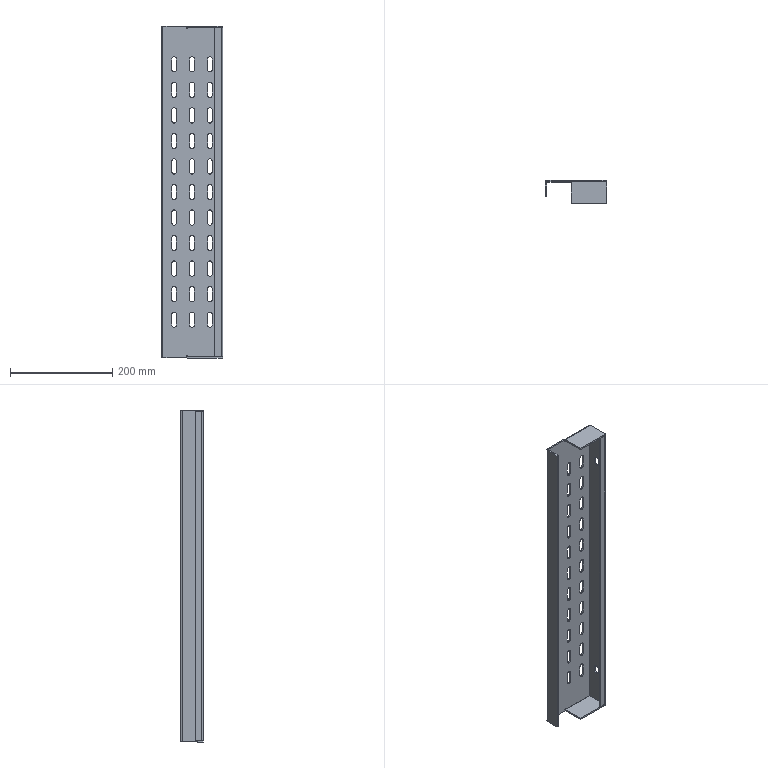Part | SolidWorks | 1 solid | 198 faces | box 120 x 45 x 650 mm | volume 377933 mm3 | plane 116 | cylinder 82 | commonest cylinder face diameters 9 x66 0.2 x5 6.2 x5 13 x4 6 x2